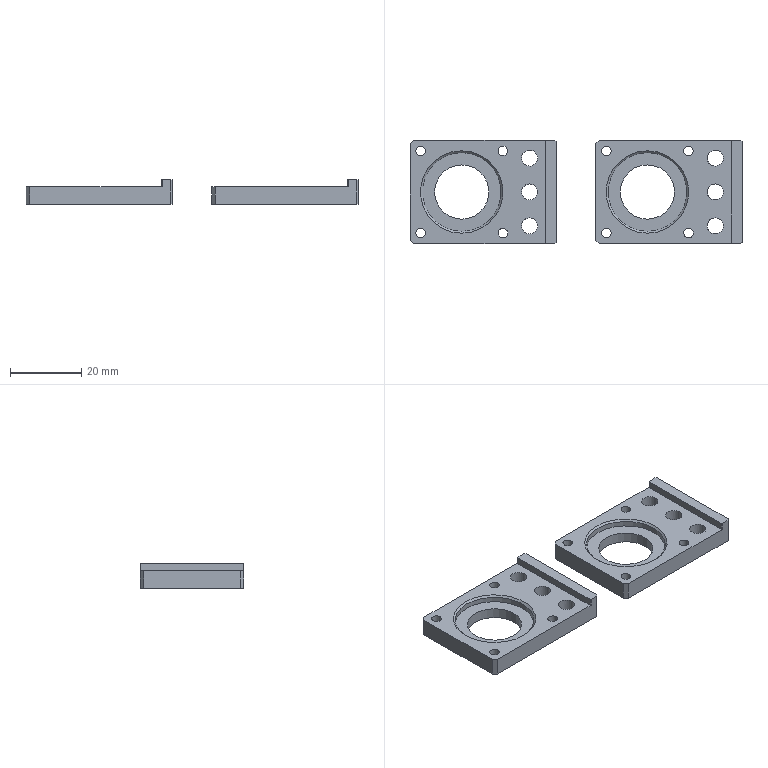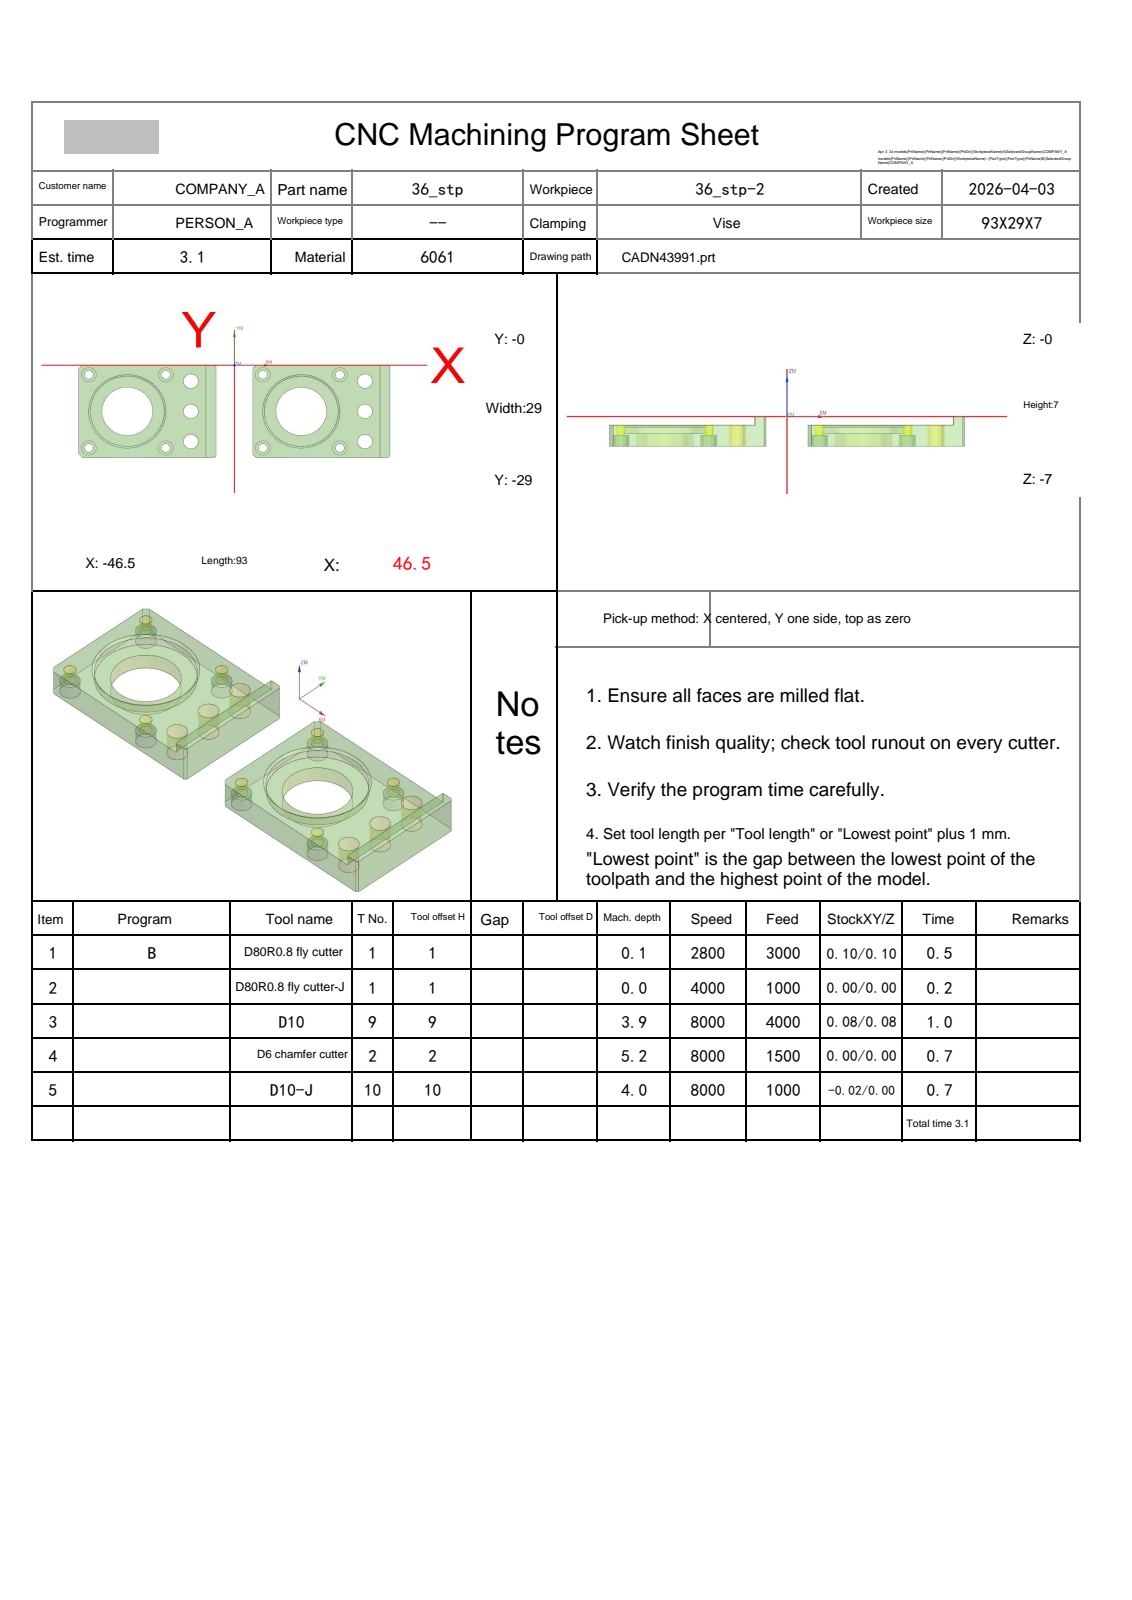NC program | NX | posted by the shop | part box 93 x 29 x 7 mm
Whole program:
%
O0001
(Machine time: 4.10 MIN)
(===Total Tool:4===)
(T1=D80R0.8 fly cutter D=80.  R=0.8  D-  H01 Z=0.    )
(T9=D10     D=10.  R=0.   D-  H09 Z=-3.92 )
(T2=D6 chamfer cutter   D=6.   R=0.   D-  H02 Z=-5.2  )
(T10=D10-J  D=10.  R=0.   D10 H10 Z=-4.   )
G80 G90 G17 G49 G40
G91 G28 Z0
M01
N1 T01 M06
(D80R0.8 fly cutter  D=80. R=0.8 H=01 ce=0.10 di=0.10)
G00 G90 G54 X-98.597 Y-14.5 M03 S2800
G43 H01 Z20.
M08
Z4.517
G01 Z2.517 F3000.
X-86.597
X86.597
X98.597
Z4.517
G00 X-98.597
Z4.033
G01 Z2.033
X-86.597
X86.597
X98.597
Z4.033
G00 X-98.597
Z3.55
G01 Z1.55
X-86.597
X86.597
X98.597
Z3.55
G00 X-98.597
Z3.067
G01 Z1.067
X-86.597
X86.597
X98.597
Z3.067
G00 Z20.
X-98.597
Z2.583
G01 Z.583
X-86.597
X86.597
X98.597
Z2.583
G00 Z20.
X-98.597
Z2.1
G01 Z.1
X-86.597
X86.597
X98.597
Z2.1
G00 Z20.
G91 G28 Z0.0
M05
M09
G91 G28 Z0.0
M01
N2 T01 M06
(D80R0.8 fly cutter-J  D=80. R=0.8 H=01 ce=0.00 di=0.00)
G00 G90 G54 X-98.499 Y-14.5 M03 S4000
G43 H01 Z20.
M08
Z2.
G01 Z0.0 F1000.
X-86.499
X86.499
X98.499
Z2.
G00 Z20.
G91 G28 Z0.0
M05
M09
G91 G28 Z0.0
M01
N3 T09 M06
(D10  D=10. R=0. H=09 ce=0.10 di=0.10)
G00 G90 G54 X19. Y-37. M03 S8000
G43 H09 Z12.8
M08
Z1.025
G01 Z-.475 F4000.
Y-33.9
X4.47
X4.18 Y-33.61
X-3.579 Y-33.791
X-.4 Y-30.612
Y1.612
X-3.579 Y4.791
X4.18 Y4.61
X4.47 Y4.9
X41.388
X38.4 Y1.912
Y-30.912
X41.388 Y-33.9
X22.035
G02 X21.203 Y-33.455 I0.0 J1.
G01 X16.797 Y-26.845
G03 X15.965 Y-26.4 I-.832 J-.555
G01 X8.097
G02 X7.1 Y-25.403 I.003 J1.
G01 Y-3.597
G02 X8.097 Y-2.6 I1. J-.003
G01 X29.903
G02 X30.9 Y-3.597 I-.003 J-1.
G01 Y-25.403
G02 X29.903 Y-26.4 I-1. J.003
G01 X22.035
G02 X21.203 Y-25.955 I0.0 J1.
G01 X16.797 Y-19.345
G03 X15.965 Y-18.9 I-.832 J-.555
G01 X15.597
G02 X14.6 Y-17.903 I.003 J1.
G01 Y-11.097
G02 X15.597 Y-10.1 I1. J-.003
G01 X22.403
G02 X23.4 Y-11.097 I-.003 J-1.
G01 Y-17.903
G02 X22.403 Y-18.9 I-1. J.003
G01 X19.
X18.5
Y-21.9
Z1.025
G00 X19. Y-37.
Z.55
G01 Z-.95
Y-33.9
X4.47
X4.18 Y-33.61
X-3.579 Y-33.791
X-.4 Y-30.612
Y1.612
X-3.579 Y4.791
X4.18 Y4.61
X4.47 Y4.9
X41.388
X38.4 Y1.912
Y-30.912
X41.388 Y-33.9
X22.035
G02 X21.203 Y-33.455 I0.0 J1.
G01 X16.797 Y-26.845
G03 X15.965 Y-26.4 I-.832 J-.555
G01 X8.097
G02 X7.1 Y-25.403 I.003 J1.
G01 Y-3.597
G02 X8.097 Y-2.6 I1. J-.003
G01 X29.903
G02 X30.9 Y-3.597 I-.003 J-1.
G01 Y-25.403
G02 X29.903 Y-26.4 I-1. J.003
G01 X22.035
G02 X21.203 Y-25.955 I0.0 J1.
G01 X16.797 Y-19.345
G03 X15.965 Y-18.9 I-.832 J-.555
G01 X15.597
G02 X14.6 Y-17.903 I.003 J1.
G01 Y-11.097
G02 X15.597 Y-10.1 I1. J-.003
G01 X22.403
G02 X23.4 Y-11.097 I-.003 J-1.
G01 Y-17.903
G02 X22.403 Y-18.9 I-1. J.003
G01 X19.
X18.5
Y-21.9
Z.55
G00 X19. Y-37.
Z.075
G01 Z-1.425
Y-33.9
X4.47
X4.18 Y-33.61
X-3.579 Y-33.791
X-.4 Y-30.612
Y1.612
X-3.579 Y4.791
X4.18 Y4.61
X4.47 Y4.9
X41.388
X38.4 Y1.912
Y-30.912
X41.388 Y-33.9
X22.035
G02 X21.203 Y-33.455 I0.0 J1.
G01 X16.797 Y-26.845
G03 X15.965 Y-26.4 I-.832 J-.555
G01 X8.097
G02 X7.1 Y-25.403 I.003 J1.
G01 Y-3.597
G02 X8.097 Y-2.6 I1. J-.003
G01 X29.903
G02 X30.9 Y-3.597 I-.003 J-1.
G01 Y-25.403
G02 X29.903 Y-26.4 I-1. J.003
G01 X22.035
G02 X21.203 Y-25.955 I0.0 J1.
G01 X16.797 Y-19.345
G03 X15.965 Y-18.9 I-.832 J-.555
G01 X15.597
G02 X14.6 Y-17.903 I.003 J1.
G01 Y-11.097
G02 X15.597 Y-10.1 I1. J-.003
G01 X22.403
G02 X23.4 Y-11.097 I-.003 J-1.
G01 Y-17.903
G02 X22.403 Y-18.9 I-1. J.003
G01 X19.
X18.5
Y-21.9
Z.075
G00 X19. Y-37.
Z-.4
G01 Z-1.9
Y-33.9
X4.47
X4.18 Y-33.61
X-3.579 Y-33.791
X-.4 Y-30.612
Y1.612
X-3.579 Y4.791
X4.18 Y4.61
X4.47 Y4.9
X41.388
X38.4 Y1.912
Y-30.912
X41.388 Y-33.9
X22.035
G02 X21.203 Y-33.455 I0.0 J1.
G01 X16.797 Y-26.845
G03 X15.965 Y-26.4 I-.832 J-.555
G01 X8.097
G02 X7.1 Y-25.403 I.003 J1.
G01 Y-3.597
G02 X8.097 Y-2.6 I1. J-.003
G01 X29.903
G02 X30.9 Y-3.597 I-.003 J-1.
G01 Y-25.403
G02 X29.903 Y-26.4 I-1. J.003
G01 X22.035
G02 X21.203 Y-25.955 I0.0 J1.
G01 X16.797 Y-19.345
G03 X15.965 Y-18.9 I-.832 J-.555
G01 X15.597
G02 X14.6 Y-17.903 I.003 J1.
G01 Y-11.097
G02 X15.597 Y-10.1 I1. J-.003
G01 X22.403
G02 X23.4 Y-11.097 I-.003 J-1.
G01 Y-17.903
G02 X22.403 Y-18.9 I-1. J.003
G01 X19.
X18.5
Y-21.9
Z-.4
G00 Z12.8
X-32.5 Y-37.
Z1.025
G01 Z-.475
Y-33.9
X-47.53
X-48.965 Y-32.465
X-51.4 Y-30.03
Y1.03
X-47.53 Y4.9
X-10.612
X-13.6 Y1.912
Y-30.912
X-10.612 Y-33.9
X-29.465
G02 X-30.297 Y-33.455 I0.0 J1.
G01 X-34.703 Y-26.845
G03 X-35.535 Y-26.4 I-.832 J-.555
G01 X-42.903
G02 X-43.9 Y-25.403 I.003 J1.
G01 Y-3.597
G02 X-42.903 Y-2.6 I1. J-.003
G01 X-22.097
G02 X-21.1 Y-3.597 I-.003 J-1.
G01 Y-25.403
G02 X-22.097 Y-26.4 I-1. J.003
G01 X-29.465
G02 X-30.297 Y-25.955 I0.0 J1.
G01 X-34.707 Y-19.34
G03 X-35.469 Y-18.898 I-.832 J-.555
G02 X-36.4 Y-17.903 I.069 J.998
G01 Y-11.097
G02 X-35.403 Y-10.1 I1. J-.003
G01 X-29.597
G02 X-28.6 Y-11.097 I-.003 J-1.
G01 Y-17.903
G02 X-29.597 Y-18.9 I-1. J.003
G01 X-32.5
X-33.
Y-21.9
Z1.025
G00 X-32.5 Y-37.
Z.55
G01 Z-.95
Y-33.9
X-47.53
X-48.965 Y-32.465
X-51.4 Y-30.03
Y1.03
X-47.53 Y4.9
X-10.612
X-13.6 Y1.912
Y-30.912
X-10.612 Y-33.9
X-29.465
G02 X-30.297 Y-33.455 I0.0 J1.
G01 X-34.703 Y-26.845
G03 X-35.535 Y-26.4 I-.832 J-.555
G01 X-42.903
G02 X-43.9 Y-25.403 I.003 J1.
G01 Y-3.597
G02 X-42.903 Y-2.6 I1. J-.003
G01 X-22.097
G02 X-21.1 Y-3.597 I-.003 J-1.
G01 Y-25.403
G02 X-22.097 Y-26.4 I-1. J.003
G01 X-29.465
G02 X-30.297 Y-25.955 I0.0 J1.
G01 X-34.707 Y-19.34
G03 X-35.469 Y-18.898 I-.832 J-.555
G02 X-36.4 Y-17.903 I.069 J.998
G01 Y-11.097
G02 X-35.403 Y-10.1 I1. J-.003
G01 X-29.597
G02 X-28.6 Y-11.097 I-.003 J-1.
G01 Y-17.903
G02 X-29.597 Y-18.9 I-1. J.003
G01 X-32.5
X-33.
Y-21.9
Z.55
G00 X-32.5 Y-37.
Z.075
G01 Z-1.425
Y-33.9
X-47.53
X-48.965 Y-32.465
X-51.4 Y-30.03
Y1.03
X-47.53 Y4.9
X-10.612
X-13.6 Y1.912
Y-30.912
X-10.612 Y-33.9
X-29.465
G02 X-30.297 Y-33.455 I0.0 J1.
G01 X-34.703 Y-26.845
G03 X-35.535 Y-26.4 I-.832 J-.555
G01 X-42.903
G02 X-43.9 Y-25.403 I.003 J1.
G01 Y-3.597
G02 X-42.903 Y-2.6 I1. J-.003
G01 X-22.097
G02 X-21.1 Y-3.597 I-.003 J-1.
G01 Y-25.403
G02 X-22.097 Y-26.4 I-1. J.003
G01 X-29.465
G02 X-30.297 Y-25.955 I0.0 J1.
G01 X-34.707 Y-19.34
G03 X-35.469 Y-18.898 I-.832 J-.555
G02 X-36.4 Y-17.903 I.069 J.998
G01 Y-11.097
G02 X-35.403 Y-10.1 I1. J-.003
G01 X-29.597
G02 X-28.6 Y-11.097 I-.003 J-1.
G01 Y-17.903
G02 X-29.597 Y-18.9 I-1. J.003
G01 X-32.5
X-33.
Y-21.9
Z.075
G00 X-32.5 Y-37.
Z-.4
G01 Z-1.9
Y-33.9
X-47.53
X-48.965 Y-32.465
X-51.4 Y-30.03
Y1.03
X-47.53 Y4.9
X-10.612
X-13.6 Y1.912
Y-30.912
X-10.612 Y-33.9
X-29.465
G02 X-30.297 Y-33.455 I0.0 J1.
G01 X-34.703 Y-26.845
G03 X-35.535 Y-26.4 I-.832 J-.555
G01 X-42.903
G02 X-43.9 Y-25.403 I.003 J1.
G01 Y-3.597
G02 X-42.903 Y-2.6 I1. J-.003
G01 X-22.097
G02 X-21.1 Y-3.597 I-.003 J-1.
G01 Y-25.403
G02 X-22.097 Y-26.4 I-1. J.003
G01 X-29.465
G02 X-30.297 Y-25.955 I0.0 J1.
G01 X-34.707 Y-19.34
G03 X-35.469 Y-18.898 I-.832 J-.555
G02 X-36.4 Y-17.903 I.069 J.998
G01 Y-11.097
G02 X-35.403 Y-10.1 I1. J-.003
G01 X-29.597
G02 X-28.6 Y-11.097 I-.003 J-1.
G01 Y-17.903
G02 X-29.597 Y-18.9 I-1. J.003
G01 X-32.5
X-33.
Y-21.9
Z-.4
G00 Z12.8
G00 G90 X-32. Y-14.5 M03 S6000
Z20.
Z-1.
G03 X-30. Y-16.5 I2. J0.0 F2700.
X-28. Y-14.5 I0.0 J2.
X-28. Y-14.5 Z-1.2 I-4. J0.0 F3000.
X-28. Y-14.5 Z-1.4 I-4. J0.0
X-28. Y-14.5 Z-1.6 I-4. J0.0
X-28. Y-14.5 Z-1.8 I-4. J0.0
X-28. Y-14.5 Z-2. I-4. J0.0
X-28. Y-14.5 Z-2.2 I-4. J0.0
X-28. Y-14.5 Z-2.4 I-4. J0.0
X-28. Y-14.5 Z-2.6 I-4. J0.0
X-28. Y-14.5 Z-2.8 I-4. J0.0
X-28. Y-14.5 Z-3. I-4. J0.0
X-28. Y-14.5 Z-3.2 I-4. J0.0
X-28. Y-14.5 Z-3.4 I-4. J0.0
X-28. Y-14.5 Z-3.6 I-4. J0.0
X-28. Y-14.5 Z-3.8 I-4. J0.0
X-35.236 Y-16.851 Z-3.92 I-4. J0.0
X-31.929 Y-18.536 I3.307 J2.403
X-29.608 Y-17.813 I0.0 J4.087
X-27.81 Y-14.388 I-2.364 J3.425
X-28.451 Y-12.169 I-4.161 J0.0
X-32.08 Y-10.166 I-3.629 J-2.288
X-34.284 Y-10.776 I0.0 J-4.29
X-36.447 Y-14.591 I2.284 J-3.816
X-35.867 Y-16.787 I4.447 J0.0
X-31.922 Y-19.084 I3.945 J2.24
X-29.774 Y-18.543 I0.0 J4.536
X-27.303 Y-14.409 I-2.222 J4.134
X-27.812 Y-12.283 I-4.693 J0.0
X-32.076 Y-9.667 I-4.264 J-2.167
X-34.143 Y-10.137 I0.0 J-4.783
X-36.948 Y-14.591 I2.135 J-4.454
X-36.511 Y-16.623 I4.94 J0.0
X-31.927 Y-19.583 I4.584 J2.068
X-29.965 Y-19.185 I0.0 J5.029
X-26.802 Y-14.41 I-2.023 J4.775
X-27.167 Y-12.498 I-5.186 J0.0
X-32.071 Y-9.167 I-4.904 J-1.944
X-33.901 Y-9.495 I0.0 J-5.275
X-37.449 Y-14.59 I1.884 J-5.095
X-37.154 Y-16.355 I5.432 J0.0
X-31.932 Y-20.082 I5.222 J1.795
X-30.259 Y-19.823 I0.0 J5.522
X-26.301 Y-14.411 I-1.72 J5.412
X-26.529 Y-12.817 I-5.679 J0.0
X-32.104 Y-8.64 I-5.574 J-1.63
X-33.677 Y-8.857 I0.0 J-5.808
X-37.967 Y-14.521 I1.594 J-5.664
X-37.782 Y-15.985 I5.885 J0.0
X-32. Y-20.47 I5.782 J1.485
X-26.03 Y-14.5 I0.0 J5.97
X-32. Y-8.53 I-5.97 J0.0
X-37.97 Y-14.5 I0.0 J-5.97
X-37.638 Y-16.463 I5.97 J0.0
X-34.819 Y-18.467 I2.819 J.982
X-31.834 Y-15.482 I0.0 J2.985
X-32. Y-14.5 I-2.985 J0.0
G00 Z20.
X20.
Z-1.
G03 X22. Y-16.5 I2. J0.0 F2700.
X24. Y-14.5 I0.0 J2.
X24. Y-14.5 Z-1.2 I-4. J0.0 F3000.
X24. Y-14.5 Z-1.4 I-4. J0.0
X24. Y-14.5 Z-1.6 I-4. J0.0
X24. Y-14.5 Z-1.8 I-4. J0.0
X24. Y-14.5 Z-2. I-4. J0.0
X24. Y-14.5 Z-2.2 I-4. J0.0
X24. Y-14.5 Z-2.4 I-4. J0.0
X24. Y-14.5 Z-2.6 I-4. J0.0
X24. Y-14.5 Z-2.8 I-4. J0.0
X24. Y-14.5 Z-3. I-4. J0.0
X24. Y-14.5 Z-3.2 I-4. J0.0
X24. Y-14.5 Z-3.4 I-4. J0.0
X24. Y-14.5 Z-3.6 I-4. J0.0
X24. Y-14.5 Z-3.8 I-4. J0.0
X16.764 Y-16.851 Z-3.92 I-4. J0.0
X20.071 Y-18.536 I3.307 J2.403
X22.392 Y-17.813 I0.0 J4.087
X24.19 Y-14.388 I-2.364 J3.425
X23.549 Y-12.169 I-4.161 J0.0
X19.92 Y-10.166 I-3.629 J-2.288
X17.716 Y-10.776 I0.0 J-4.29
X15.553 Y-14.591 I2.284 J-3.816
X16.133 Y-16.787 I4.447 J0.0
X20.078 Y-19.084 I3.945 J2.24
X22.226 Y-18.543 I0.0 J4.536
X24.697 Y-14.409 I-2.222 J4.134
X24.188 Y-12.283 I-4.693 J0.0
X19.924 Y-9.667 I-4.264 J-2.167
X17.857 Y-10.137 I0.0 J-4.783
X15.052 Y-14.591 I2.135 J-4.454
X15.489 Y-16.623 I4.94 J0.0
X20.073 Y-19.583 I4.584 J2.068
X22.035 Y-19.185 I0.0 J5.029
X25.198 Y-14.41 I-2.023 J4.775
X24.833 Y-12.498 I-5.186 J0.0
X19.929 Y-9.167 I-4.904 J-1.944
X18.099 Y-9.495 I0.0 J-5.275
X14.551 Y-14.59 I1.884 J-5.095
X14.846 Y-16.355 I5.432 J0.0
X20.068 Y-20.082 I5.222 J1.795
X21.741 Y-19.823 I0.0 J5.522
X25.699 Y-14.411 I-1.72 J5.412
X25.471 Y-12.817 I-5.679 J0.0
X19.896 Y-8.64 I-5.574 J-1.63
X18.323 Y-8.857 I0.0 J-5.808
X14.033 Y-14.521 I1.594 J-5.664
X14.218 Y-15.985 I5.885 J0.0
X20. Y-20.47 I5.782 J1.485
X25.97 Y-14.5 I0.0 J5.97
X20. Y-8.53 I-5.97 J0.0
X14.03 Y-14.5 I0.0 J-5.97
X14.362 Y-16.463 I5.97 J0.0
X17.181 Y-18.467 I2.819 J.982
X20.166 Y-15.482 I0.0 J2.985
X20. Y-14.5 I-2.985 J0.0
G00 Z20.
G91 G28 Z0.0
M05
M09
G91 G28 Z0.0
M01
N4 T02 M06
(D6 chamfer cutter  D=6. R=0. H=02 ce=0.00 di=0.08)
G00 G90 G54 X8.5 Y-26. M03 S8000
G43 H02 Z20.
M08
G98 G81 X8.5 Y-26. Z-3.65 R1. F1000.
X31.5
Y-3.
X8.5
X-20.5
Y-26.
X-43.5
Y-3.
G80
G00 Z20.
G00 G90 X-13. Y-5. M03 S8000
Z20.
G98 G81 X-13. Y-5. Z-4.55 R1. F1000.
Y-14.5
Y-24.
X39.
Y-14.5
Y-5.
G80
G00 Z20.
G00 G90 X-33.2 Y-23.571 M03 S6500
Z20.
Z-1.7
G01 Z-3.2 F1500.
Y-23.65
G03 X-32. Y-24.85 I1.2 J0.0
X-21.65 Y-14.5 I0.0 J10.35
X-32. Y-4.15 I-10.35 J0.0
X-42.35 Y-14.5 I0.0 J-10.35
X-32. Y-24.85 I10.35 J0.0
X-31.6 Y-24.842 I0.0 J10.35
X-30.446 Y-23.643 I-.046 J1.199
G01 X-30.447 Y-23.597
X-30.45 Y-23.518
Z-1.7
G00 Z20.
X18.8 Y-23.571
Z-1.7
G01 Z-3.2
Y-23.65
G03 X20. Y-24.85 I1.2 J0.0
X30.338 Y-15.006 I0.0 J10.35
X30.35 Y-14.5 I-10.338 J.506
X20. Y-4.15 I-10.35 J0.0
X9.65 Y-14.5 I0.0 J-10.35
X20. Y-24.85 I10.35 J0.0
X20.4 Y-24.842 I0.0 J10.35
X21.554 Y-23.643 I-.046 J1.199
G01 X21.553 Y-23.597
X21.55 Y-23.518
Z-1.7
G00 Z20.
G00 G90 X-9.727 Y-14.886 M03 S6500
Z20.
Z.172
G01 Z-1.2 F1500.
G03 X-9.527 Y-14.6 I-1.532 J1.286
G01 X-9.497 Y-14.554
X-9.5 Y-14.5
Y-.2
X-9.466 Y.059
X-9.366 Y.3
X-9.207 Y.507
X-9.007 Y.707
X-8.8 Y.866
X-8.559 Y.966
X-8.3 Y1.
X-6.
X-5.741 Y.966
X-5.5 Y.866
X-5.293 Y.707
X-4.793 Y.207
X-4.634 Y0.0
X-4.534 Y-.241
X-4.5 Y-.5
Y-28.5
X-4.534 Y-28.759
X-4.634 Y-29.
X-4.793 Y-29.207
X-5.293 Y-29.707
X-5.5 Y-29.866
X-5.741 Y-29.966
X-6. Y-30.
X-8.3
X-8.559 Y-29.966
X-8.8 Y-29.866
X-9.007 Y-29.707
X-9.207 Y-29.507
X-9.366 Y-29.3
X-9.466 Y-29.059
X-9.5 Y-28.8
Y-14.5
X-9.497 Y-14.446
X-9.527 Y-14.4
G03 X-9.727 Y-14.114 I-1.732 J-1.
G01 Z.172
G00 Z10.
X42.273 Y-14.886
Z.172
G01 Z-1.2
G03 X42.473 Y-14.6 I-1.532 J1.286
G01 X42.503 Y-14.554
X42.5 Y-14.5
Y-.2
X42.534 Y.059
X42.634 Y.3
X42.793 Y.507
X42.993 Y.707
X43.2 Y.866
X43.441 Y.966
X43.7 Y1.
X46.
X46.259 Y.966
X46.5 Y.866
X46.707 Y.707
X47.207 Y.207
X47.366 Y0.0
X47.466 Y-.241
X47.5 Y-.5
Y-28.5
X47.466 Y-28.759
X47.366 Y-29.
X47.207 Y-29.207
X46.707 Y-29.707
X46.5 Y-29.866
X46.259 Y-29.966
X46. Y-30.
X43.7
X43.441 Y-29.966
X43.2 Y-29.866
X42.993 Y-29.707
X42.793 Y-29.507
X42.634 Y-29.3
X42.534 Y-29.059
X42.5 Y-28.8
Y-14.5
X42.503 Y-14.446
X42.473 Y-14.4
G03 X42.273 Y-14.114 I-1.732 J-1.
G01 Z.172
G00 Z10.
X40.621 Y-30.091
Z-1.692
G01 Z-3.2
X40.571 Y-30.04
X40.507 Y-30.011
X40.49 Y-29.993
X40.467 Y-30.
X6.5
X6.241 Y-29.966
X6. Y-29.866
X5.793 Y-29.707
X4.793 Y-28.707
X4.634 Y-28.5
X4.534 Y-28.259
X4.5 Y-28.
Y-1.
X4.534 Y-.741
X4.634 Y-.5
X4.793 Y-.293
X5.793 Y.707
X6. Y.866
X6.241 Y.966
X6.5 Y1.
X40.467
X40.49 Y.993
X40.507 Y1.011
X40.571 Y1.04
X40.621 Y1.091
Z-1.692
G00 Z10.
X40.065 Y-24.407
Z-1.706
G01 Z-3.2
G03 X40.234 Y-24.102 I-1.658 J1.118
G01 X40.259 Y-24.054
X40.25 Y-24.
G03 X39. Y-22.75 I-1.25 J0.0
X37.75 Y-24. I0.0 J-1.25
X39. Y-25.25 I1.25 J0.0
X40.223 Y-24.26 I0.0 J1.25
G01 X40.25 Y-24.
X40.259 Y-23.946
X40.234 Y-23.898
G03 X40.065 Y-23.593 I-1.827 J-.813
G01 Z-1.706
G00 Z.55
X31.725 Y-26.335
Z-1.54
G01 Z-3.2
G03 X31.843 Y-26.083 I-1.386 J.8
G01 X31.862 Y-26.043
X31.85 Y-26.
G03 X31.5 Y-25.65 I-.35 J0.0
X31.15 Y-26. I0.0 J-.35
X31.5 Y-26.35 I.35 J0.0
X31.829 Y-26.12 I0.0 J.35
G01 X31.85 Y-26.
X31.862 Y-25.957
X31.843 Y-25.917
G03 X31.725 Y-25.665 I-1.504 J-.547
G01 Z-1.54
G00 Z10.
X40.065 Y-14.907
Z-1.706
G01 Z-3.2
G03 X40.234 Y-14.602 I-1.658 J1.118
G01 X40.259 Y-14.554
X40.25 Y-14.5
G03 X39. Y-13.25 I-1.25 J0.0
X37.75 Y-14.5 I0.0 J-1.25
X39. Y-15.75 I1.25 J0.0
X40.223 Y-14.76 I0.0 J1.25
G01 X40.25 Y-14.5
X40.259 Y-14.446
X40.234 Y-14.398
G03 X40.065 Y-14.093 I-1.827 J-.813
G01 Z-1.706
G00 Z.55
Y-5.407
Z-1.706
G01 Z-3.2
G03 X40.234 Y-5.102 I-1.658 J1.118
G01 X40.259 Y-5.054
X40.25 Y-5.
G03 X39. Y-3.75 I-1.25 J0.0
X37.75 Y-5. I0.0 J-1.25
X39. Y-6.25 I1.25 J0.0
X40.223 Y-5.26 I0.0 J1.25
G01 X40.25 Y-5.
X40.259 Y-4.946
X40.234 Y-4.898
G03 X40.065 Y-4.593 I-1.827 J-.813
G01 Z-1.706
G00 Z.55
X31.725 Y-3.335
Z-1.54
G01 Z-3.2
G03 X31.843 Y-3.083 I-1.386 J.8
G01 X31.862 Y-3.043
X31.85 Y-3.
G03 X31.5 Y-2.65 I-.35 J0.0
X31.15 Y-3. I0.0 J-.35
X31.5 Y-3.35 I.35 J0.0
X31.829 Y-3.12 I0.0 J.35
G01 X31.85 Y-3.
X31.862 Y-2.957
X31.843 Y-2.917
G03 X31.725 Y-2.665 I-1.504 J-.547
G01 Z-1.54
G00 Z10.
X8.725 Y-3.335
Z-1.54
G01 Z-3.2
G03 X8.843 Y-3.083 I-1.386 J.8
G01 X8.862 Y-3.043
X8.85 Y-3.
G03 X8.5 Y-2.65 I-.35 J0.0
X8.15 Y-3. I0.0 J-.35
X8.5 Y-3.35 I.35 J0.0
X8.829 Y-3.12 I0.0 J.35
G01 X8.85 Y-3.
X8.862 Y-2.957
X8.843 Y-2.917
G03 X8.725 Y-2.665 I-1.504 J-.547
G01 Z-1.54
G00 Z10.
Y-26.335
Z-1.54
G01 Z-3.2
G03 X8.843 Y-26.083 I-1.386 J.8
G01 X8.862 Y-26.043
X8.85 Y-26.
G03 X8.5 Y-25.65 I-.35 J0.0
X8.15 Y-26. I0.0 J-.35
X8.5 Y-26.35 I.35 J0.0
X8.829 Y-26.12 I0.0 J.35
G01 X8.85 Y-26.
X8.862 Y-25.957
X8.843 Y-25.917
G03 X8.725 Y-25.665 I-1.504 J-.547
G01 Z-1.54
G00 Z10.
X-11.379 Y-30.091
Z-1.692
G01 Z-3.2
X-11.429 Y-30.04
X-11.493 Y-30.011
X-11.51 Y-29.993
X-11.533 Y-30.
X-45.5
X-45.759 Y-29.966
X-46. Y-29.866
X-46.207 Y-29.707
X-47.207 Y-28.707
X-47.366 Y-28.5
X-47.466 Y-28.259
X-47.5 Y-28.
Y-1.
X-47.466 Y-.741
X-47.366 Y-.5
X-47.207 Y-.293
X-46.207 Y.707
X-46. Y.866
X-45.759 Y.966
X-45.5 Y1.
X-11.533
X-11.51 Y.993
X-11.493 Y1.011
X-11.429 Y1.04
X-11.379 Y1.091
Z-1.692
G00 Z10.
X-11.935 Y-24.407
Z-1.706
G01 Z-3.2
G03 X-11.766 Y-24.102 I-1.658 J1.118
G01 X-11.741 Y-24.054
X-11.75 Y-24.
G03 X-13. Y-22.75 I-1.25 J0.0
X-14.25 Y-24. I0.0 J-1.25
X-13. Y-25.25 I1.25 J0.0
X-11.777 Y-24.26 I0.0 J1.25
G01 X-11.75 Y-24.
X-11.741 Y-23.946
X-11.766 Y-23.898
G03 X-11.935 Y-23.593 I-1.827 J-.813
G01 Z-1.706
G00 Z.55
X-20.275 Y-26.335
Z-1.54
G01 Z-3.2
G03 X-20.157 Y-26.083 I-1.386 J.8
G01 X-20.138 Y-26.043
X-20.15 Y-26.
G03 X-20.5 Y-25.65 I-.35 J0.0
X-20.85 Y-26. I0.0 J-.35
X-20.5 Y-26.35 I.35 J0.0
X-20.171 Y-26.12 I0.0 J.35
G01 X-20.15 Y-26.
X-20.138 Y-25.957
X-20.157 Y-25.917
G03 X-20.275 Y-25.665 I-1.504 J-.547
G01 Z-1.54
G00 Z10.
X-11.935 Y-14.907
Z-1.706
G01 Z-3.2
G03 X-11.766 Y-14.602 I-1.658 J1.118
G01 X-11.741 Y-14.554
X-11.75 Y-14.5
G03 X-13. Y-13.25 I-1.25 J0.0
X-14.25 Y-14.5 I0.0 J-1.25
X-13. Y-15.75 I1.25 J0.0
X-11.777 Y-14.76 I0.0 J1.25
G01 X-11.75 Y-14.5
X-11.741 Y-14.446
X-11.766 Y-14.398
G03 X-11.935 Y-14.093 I-1.827 J-.813
G01 Z-1.706
G00 Z.55
Y-5.407
Z-1.706
G01 Z-3.2
G03 X-11.766 Y-5.102 I-1.658 J1.118
G01 X-11.741 Y-5.054
X-11.75 Y-5.
G03 X-13. Y-3.75 I-1.25 J0.0
X-14.25 Y-5. I0.0 J-1.25
X-13. Y-6.25 I1.25 J0.0
X-11.777 Y-5.26 I0.0 J1.25
G01 X-11.75 Y-5.
X-11.741 Y-4.946
X-11.766 Y-4.898
G03 X-11.935 Y-4.593 I-1.827 J-.813
G01 Z-1.706
G00 Z.55
X-20.275 Y-3.335
Z-1.54
G01 Z-3.2
G03 X-20.157 Y-3.083 I-1.386 J.8
G01 X-20.138 Y-3.043
X-20.15 Y-3.
G03 X-20.5 Y-2.65 I-.35 J0.0
X-20.85 Y-3. I0.0 J-.35
X-20.5 Y-3.35 I.35 J0.0
X-20.171 Y-3.12 I0.0 J.35
G01 X-20.15 Y-3.
X-20.138 Y-2.957
X-20.157 Y-2.917
G03 X-20.275 Y-2.665 I-1.504 J-.547
G01 Z-1.54
G00 Z10.
X-43.275 Y-3.335
Z-1.54
G01 Z-3.2
G03 X-43.157 Y-3.083 I-1.386 J.8
G01 X-43.138 Y-3.043
X-43.15 Y-3.
G03 X-43.5 Y-2.65 I-.35 J0.0
X-43.85 Y-3. I0.0 J-.35
X-43.5 Y-3.35 I.35 J0.0
X-43.171 Y-3.12 I0.0 J.35
G01 X-43.15 Y-3.
X-43.138 Y-2.957
X-43.157 Y-2.917
G03 X-43.275 Y-2.665 I-1.504 J-.547
G01 Z-1.54
G00 Z10.
Y-26.335
Z-1.54
G01 Z-3.2
G03 X-43.157 Y-26.083 I-1.386 J.8
G01 X-43.138 Y-26.043
X-43.15 Y-26.
G03 X-43.5 Y-25.65 I-.35 J0.0
X-43.85 Y-26. I0.0 J-.35
X-43.5 Y-26.35 I.35 J0.0
X-43.171 Y-26.12 I0.0 J.35
G01 X-43.15 Y-26.
X-43.138 Y-25.957
X-43.157 Y-25.917
G03 X-43.275 Y-25.665 I-1.504 J-.547
G01 Z-1.54
G00 Z10.
X-25.606 Y-14.897
Z-3.794
G01 Z-5.2
G03 X-25.422 Y-14.601 I-1.597 J1.204
G01 X-25.394 Y-14.554
X-25.4 Y-14.5
G03 X-32. Y-7.9 I-6.6 J0.0
X-38.6 Y-14.5 I0.0 J-6.6
X-32. Y-21.1 I6.6 J0.0
X-25.4 Y-14.5 I0.0 J6.6
G01 X-25.394 Y-14.446
X-25.422 Y-14.399
G03 X-25.606 Y-14.103 I-1.782 J-.908
G01 Z-3.793
G00 Z10.
X26.394 Y-14.897
Z-3.794
G01 Z-5.2
G03 X26.578 Y-14.601 I-1.597 J1.204
G01 X26.606 Y-14.554
X26.6 Y-14.5
G03 X20. Y-7.9 I-6.6 J0.0
X13.4 Y-14.5 I0.0 J-6.6
X20. Y-21.1 I6.6 J0.0
X26.6 Y-14.5 I0.0 J6.6
G01 X26.606 Y-14.446
X26.578 Y-14.399
G03 X26.394 Y-14.103 I-1.782 J-.908
G01 Z-3.793
G00 Z20.
G91 G28 Z0.0
M05
M09
G91 G28 Z0.0
M01
N5 T10 M06
(D10-J  D=10. R=0. H=10 ce=0.40 di=0.00)
G00 G90 G54 X-52.311 Y-32. M03 S8000
G43 H10 Z12.8
M08
Z-.5
G01 Z-2. F1000.
X-45.9
G03 X-43.9 Y-30. I0.0 J2.
G01 Y.1
G02 X-43. Y1. I.9 J0.0
G01 X-39.9
G02 X-38.9 Y0.0 I0.0 J-1.
G01 Y-29.1
G03 X-38. Y-30. I.9 J0.0
G01 X-34.9
G03 X-33.9 Y-29. I0.0 J1.
G01 Y.1
G02 X-33. Y1. I.9 J0.0
G01 X-29.9
G02 X-28.9 Y0.0 I0.0 J-1.
G01 Y-29.1
G03 X-28. Y-30. I.9 J0.0
G01 X-24.9
G03 X-23.9 Y-29. I0.0 J1.
G01 Y0.0
G02 X-22.9 Y1. I1. J0.0
G01 X-19.8
G02 X-18.9 Y.1 I0.0 J-.9
G01 Y-29.226
G03 X-18.15 Y-30.194 I1. J0.0
G01 X-15.15 Y-30.968
G03 X-14.9 Y-31. I.25 J.968
X-13.9 Y-30. I0.0 J1.
G01 Y1.
G03 X-15.9 Y3. I-2. J0.0
G01 Y7.
Z-.5
G00 Z12.8
G00 G90 X6.1 Y-36. M03 S8000
Z12.8
Z-.5
G01 Z-2. F1000.
Y-32.
G03 X8.1 Y-30. I0.0 J2.
G01 Y.1
G02 X9. Y1. I.9 J0.0
G01 X12.1
G02 X13.1 Y0.0 I0.0 J-1.
G01 Y-29.1
G03 X14. Y-30. I.9 J0.0
G01 X17.1
G03 X18.1 Y-29. I0.0 J1.
G01 Y.1
G02 X19. Y1. I.9 J0.0
G01 X22.1
G02 X23.1 Y0.0 I0.0 J-1.
G01 Y-29.1
G03 X24. Y-30. I.9 J0.0
G01 X27.1
G03 X28.1 Y-29. I0.0 J1.
G01 Y.1
G02 X29. Y1. I.9 J0.0
G01 X32.1
G02 X33.1 Y0.0 I0.0 J-1.
G01 Y-29.226
G03 X33.85 Y-30.194 I1. J0.0
G01 X36.85 Y-30.968
G03 X37.1 Y-31. I.25 J.968
X38.1 Y-30. I0.0 J1.
G01 Y1.
G03 X36.1 Y3. I-2. J0.0
G01 Y7.
Z-.5
G00 Z12.8
G00 G90 X-9.932 Y-36.191 M03 S8000
Z12.8
Z-1.
G01 Z-2. F1000.
G41 D10
X-9.873 Y-36.
G03 X-9.785 Y-35.414 I-1.912 J.586
X-10.371 Y-34. I-2. J0.0
G01 X-13.5 Y-30.871
Y1.871
X-10.371 Y5.
G03 X-9.785 Y6.414 I-1.414 J1.414
X-9.873 Y7. I-2. J0.0
G01 G40 X-9.932 Y7.191
Z-1.
G00 Z12.8
G00 G90 X42.064 Y-36.191 M03 S8000
Z12.8
Z-1.
G01 Z-2. F1000.
G41 D10
X42.123 Y-36.
G03 X42.212 Y-35.411 I-1.911 J.589
X41.626 Y-33.997 I-2. J0.0
G01 X38.5 Y-30.871
Y1.871
X41.629 Y5.
G03 X42.215 Y6.414 I-1.414 J1.414
X42.127 Y7. I-2. J0.0
G01 G40 X42.068 Y7.191
Z-1.
G00 Z12.8
G00 G90 X-35.345 Y-12.5 M03 S8000
Z12.8
Z-3.
G01 Z-4. F1000.
G41 D10
X-36.07
G03 X-38.07 Y-14.5 I0.0 J-2.
X-32. Y-20.57 I6.07 J0.0
X-25.93 Y-14.5 I0.0 J6.07
X-32. Y-8.43 I-6.07 J0.0
X-38.07 Y-14.5 I0.0 J-6.07
X-38.057 Y-14.9 I6.07 J0.0
X-36.061 Y-16.768 I1.996 J.132
G01 X-35.929 Y-16.764
X-35.405 Y-16.729
G40 X-35.206 Y-16.716
Z-3.
G00 Z12.8
X22. Y-11.155
Z-3.
G01 Z-4.
G41 D10
Y-10.43
G03 X20. Y-8.43 I-2. J0.0
X13.93 Y-14.5 I0.0 J-6.07
X20. Y-20.57 I6.07 J0.0
X26.07 Y-14.5 I0.0 J6.07
X20. Y-8.43 I-6.07 J0.0
X19.6 Y-8.443 I0.0 J-6.07
X17.732 Y-10.439 I.132 J-1.996
G01 X17.736 Y-10.571
X17.771 Y-11.095
G40 X17.784 Y-11.294
Z-3.
G00 Z12.8
M05
M09
G91 G28 Z0.0
G91 G28 Y0.0
M30
%